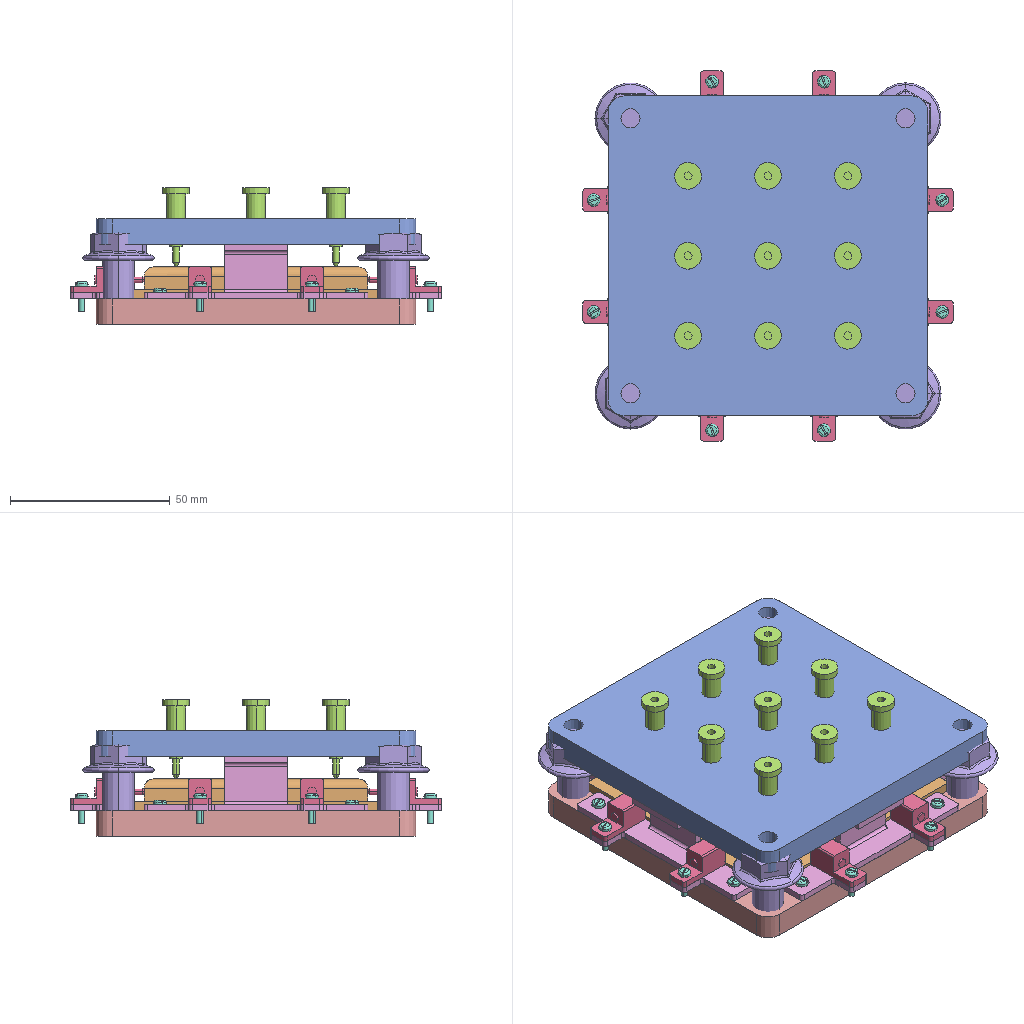Assembly | SolidWorks | 11 different items | 32 placed | box 116 x 116 x 43 mm
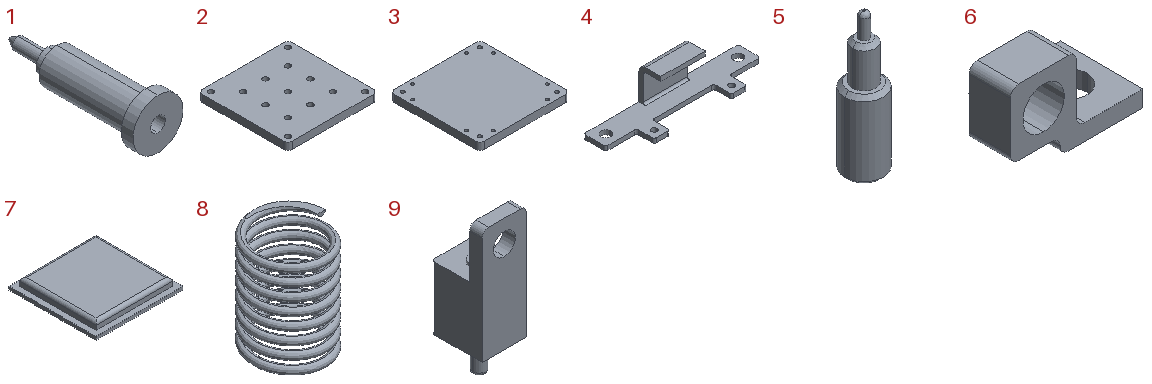Parts list (item | name | quantity | size | volume | features):
1 | - | x9 | 8.4 x 24.799 x 8.4 mm | 541.841 mm3 | features Revolution 1
2 | - | x1 | 100 x 100 x 8 mm | 76888 mm3 | features Extrusion 1
3 | - | x1 | 100 x 100 x 8 mm | 78838 mm3 | features 3DProfileFeature 2, HoleWzd 2, Extrusion 1
4 | - | x4 | 70 x 18 x 17 mm | 2429 mm3 | features Fillet 4, ICE 4, 3DProfileFeature 1, Extrusion 1, HoleWzd 1
5 | - | x1 | 5 x 5 x 18 mm | 197.687 mm3 | features ICE 3, Chamfer 1, Extrusion 1, Fillet 1
6 | - | x1 | 16 x 10 x 10 mm | 387.871 mm3 | features ICE 4, Fillet 2, Extrusion 1
7 | - | x1 | 80 x 80 x 10 mm | 52970 mm3 | features Extrusion 1, Fillet 1, ICE 1
8 | - | x4 | 8.9 x 8.9 x 12 mm | 125.858 mm3 | features ICE 2, Helix 1, Sweep 1
9 | - | x8 | 7 x 8 x 23 mm | 673.267 mm3 | features ICE 5, Fillet 3, Extrusion 1
10 | hex flange bolts-heavy grade b gb | x1 | - | - | -
11 | slotted pan head screws gb | x1 | - | - | -
Mates (type | each side: item.copy, entity, surface, feature):
Coincident | 3.1 face plane Boss-Extrude1 | 2.1 face plane Boss-Extrude1 | 2 times
Concentric | 2.1 face cylinder Boss-Extrude1 | 1.1 face cylinder Revolve1
Concentric | 3.1 face cylinder M4 Tapped Hole1 | 4.1 face cylinder Cut-Extrude1 | 2 times
Coincident | 3.1 face plane Boss-Extrude1 | 4.1 face plane Boss-Extrude1
Coincident | 3.1 face plane Boss-Extrude1 | 7.1 face plane Boss-Extrude1
Coincident | 4.2 face plane Boss-Extrude1 | 7.1 face plane Boss-Extrude1
Coincident | 4.1 face plane Boss-Extrude1 | 7.1 face plane Boss-Extrude1
Coincident | 1.1 face plane Revolve1 | 7.1 face plane Boss-Extrude2
Coincident | 2.1 face plane Boss-Extrude1 | 4.1 face plane Boss-Extrude2
Coincident | 4.1 face plane Boss-Extrude1 | 9.1 face plane Boss-Extrude1
Concentric | 4.1 face cylinder M3 Tapped Hole1 | 9.1 face cylinder Cut-Extrude1
Parallel | 4.1 face plane Boss-Extrude4 | 9.1 face plane Boss-Extrude1
Coincident | 4.1 face plane Boss-Extrude1 | 9.2 face plane Boss-Extrude1
Concentric | 4.1 face cylinder M3 Tapped Hole1 | 9.2 face cylinder Cut-Extrude1
Coincident | 4.1 face plane Boss-Extrude4 | 9.2 face plane Boss-Extrude1